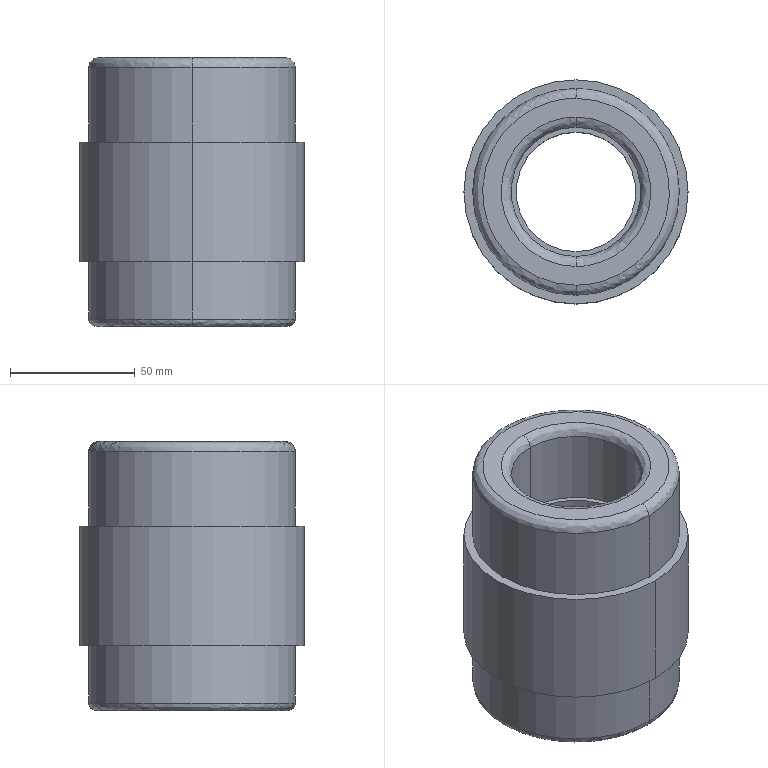Part | SolidWorks | features BaseBody 1 | 1 solid | 26 faces | box 90 x 90 x 108 mm | volume 413534 mm3 | cylinder 12 | spline 8 | plane 6 | commonest cylinder face diameters 52 x4 83 x4 48 x2 90 x2